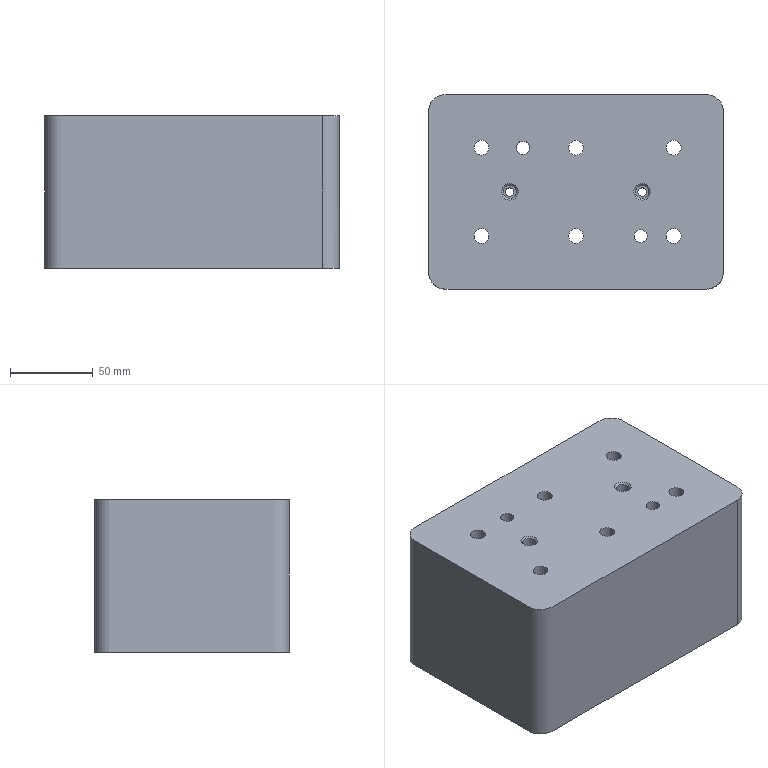Part | NX | features solid 2 | 1 solid | 45 faces | box 178.117 x 117.446 x 92.002 mm | volume 1872320 mm3 | cylinder 24 | plane 17 | spline 2 | cone 2 | commonest cylinder face diameters 9.007 x6 14.508 x6 8 x4 20 x4 5.1 x2 10.505 x2